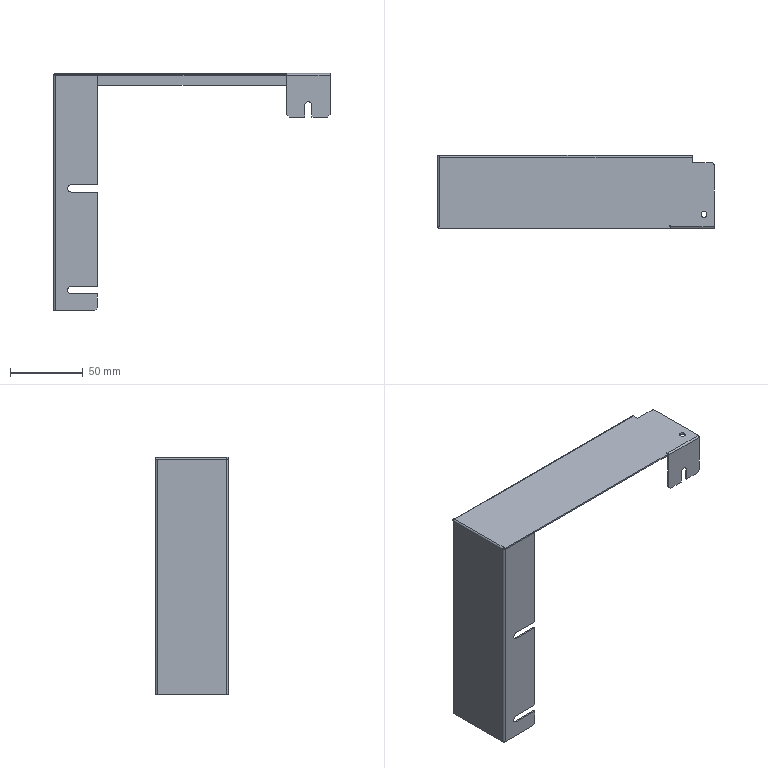Part | STEP file | 1 solid | 75 faces | box 190 x 50 x 163 mm | volume 24970 mm3 | plane 56 | cylinder 17 | spline 2 | commonest cylinder face diameters 0.2 x5 2.2 x5 5 x4 4 x3